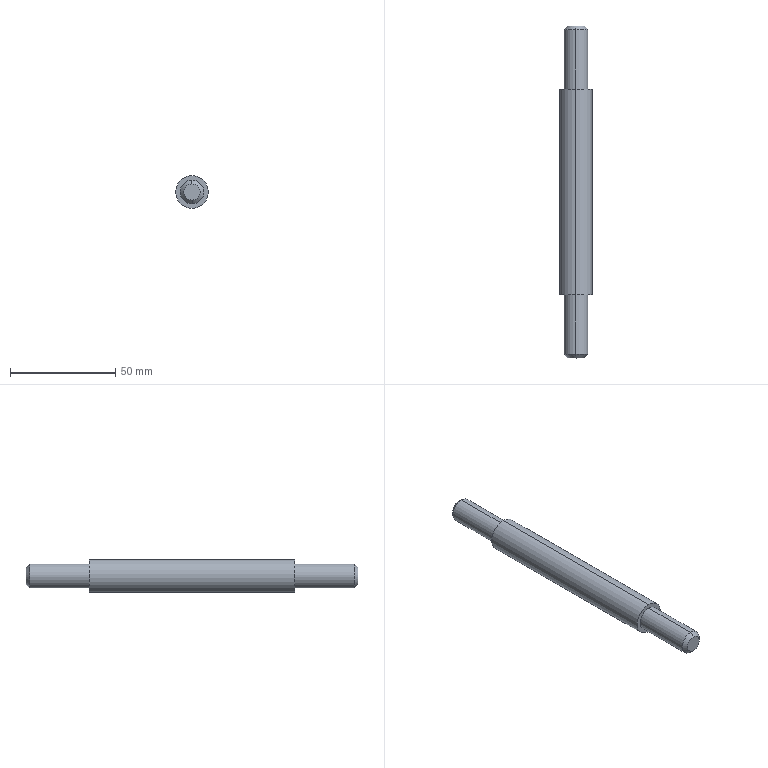Part | STEP file | Scale factor 1[3] | 1 solid | 14 faces | box 15.6 x 157.8 x 15.6 mm | volume 24713 mm3 | cylinder 6 | cone 4 | plane 4 | commonest cylinder face diameters 11.4 x4 15.6 x2
STEP:
#1=CARTESIAN_POINT('',(-699.838,-243.473,3234.6));
#2=VERTEX_POINT('',#1);
#3=CARTESIAN_POINT('',(-699.838,-243.473,3242.4));
#4=VERTEX_POINT('',#3);
#5=CARTESIAN_POINT('',(-699.838,-243.473,3238.5));
#6=DIRECTION('',(0.,1.,0.));
#7=DIRECTION('',(0.000000001,0.,-1.));
#8=AXIS2_PLACEMENT_3D('',#5,#6,#7);
#9=CIRCLE('',#8,3.9);
#10=EDGE_CURVE('',#2,#4,#9,.T.);
#11=ORIENTED_EDGE('',*,*,#10,.F.);
#12=CARTESIAN_POINT('',(-699.838,-245.273,3232.8));
#13=VERTEX_POINT('',#12);
#14=CARTESIAN_POINT('',(-699.838,-243.473,3234.6));
#15=DIRECTION('',(-0.000000001,0.7071,0.7071));
#16=VECTOR('',#15,1000.);
#17=LINE('',#14,#16);
#18=EDGE_CURVE('',#13,#2,#17,.T.);
#19=ORIENTED_EDGE('',*,*,#18,.F.);
#20=CARTESIAN_POINT('',(-699.838,-245.273,3244.2));
#21=VERTEX_POINT('',#20);
#22=CARTESIAN_POINT('',(-699.838,-245.273,3238.5));
#23=DIRECTION('',(0.,-1.,0.));
#24=DIRECTION('',(0.000000001,0.,-1.));
#25=AXIS2_PLACEMENT_3D('',#22,#23,#24);
#26=CIRCLE('',#25,5.7);
#27=EDGE_CURVE('',#21,#13,#26,.T.);
#28=ORIENTED_EDGE('',*,*,#27,.F.);
#29=CARTESIAN_POINT('',(-699.838,-243.473,3242.4));
#30=DIRECTION('',(0.000000001,0.7071,-0.7071));
#31=VECTOR('',#30,1000.);
#32=LINE('',#29,#31);
#33=EDGE_CURVE('',#21,#4,#32,.T.);
#34=ORIENTED_EDGE('',*,*,#33,.T.);
#35=EDGE_LOOP('',(#11,#19,#28,#34));
#36=FACE_OUTER_BOUND('',#35,.T.);
#37=CARTESIAN_POINT('',(-699.838,-243.473,3238.5));
#38=DIRECTION('',(0.,-1.,0.));
#39=DIRECTION('',(0.000000001,0.,-1.));
#40=AXIS2_PLACEMENT_3D('',#37,#38,#39);
#41=CONICAL_SURFACE('',#40,3.9,0.7854);
#42=ADVANCED_FACE('',(#36),#41,.T.);
#43=CARTESIAN_POINT('',(-699.838,-401.273,3242.4));
#44=VERTEX_POINT('',#43);
#45=CARTESIAN_POINT('',(-699.838,-401.273,3234.6));
#46=VERTEX_POINT('',#45);
#47=CARTESIAN_POINT('',(-699.838,-401.273,3238.5));
#48=DIRECTION('',(0.,-1.,0.));
#49=DIRECTION('',(-0.000000001,0.,1.));
#50=AXIS2_PLACEMENT_3D('',#47,#48,#49);
#51=CIRCLE('',#50,3.9);
#52=EDGE_CURVE('',#44,#46,#51,.T.);
#53=ORIENTED_EDGE('',*,*,#52,.F.);
#54=CARTESIAN_POINT('',(-699.838,-399.473,3244.2));
#55=VERTEX_POINT('',#54);
#56=CARTESIAN_POINT('',(-699.838,-401.273,3242.4));
#57=DIRECTION('',(-0.000000001,0.7071,0.7071));
#58=VECTOR('',#57,1000.);
#59=LINE('',#56,#58);
#60=EDGE_CURVE('',#44,#55,#59,.T.);
#61=ORIENTED_EDGE('',*,*,#60,.T.);
#62=CARTESIAN_POINT('',(-699.838,-399.473,3232.8));
#63=VERTEX_POINT('',#62);
#64=CARTESIAN_POINT('',(-699.838,-399.473,3238.5));
#65=DIRECTION('',(0.,1.,0.));
#66=DIRECTION('',(-0.000000001,0.,1.));
#67=AXIS2_PLACEMENT_3D('',#64,#65,#66);
#68=CIRCLE('',#67,5.7);
#69=EDGE_CURVE('',#63,#55,#68,.T.);
#70=ORIENTED_EDGE('',*,*,#69,.F.);
#71=CARTESIAN_POINT('',(-699.838,-401.273,3234.6));
#72=DIRECTION('',(0.000000001,0.7071,-0.7071));
#73=VECTOR('',#72,1000.);
#74=LINE('',#71,#73);
#75=EDGE_CURVE('',#46,#63,#74,.T.);
#76=ORIENTED_EDGE('',*,*,#75,.F.);
#77=EDGE_LOOP('',(#53,#61,#70,#76));
#78=FACE_OUTER_BOUND('',#77,.T.);
#79=CARTESIAN_POINT('',(-699.838,-401.273,3238.5));
#80=DIRECTION('',(0.,1.,0.));
#81=DIRECTION('',(-0.000000001,0.,1.));
#82=AXIS2_PLACEMENT_3D('',#79,#80,#81);
#83=CONICAL_SURFACE('',#82,3.9,0.7854);
#84=ADVANCED_FACE('',(#78),#83,.T.);
#85=ORIENTED_EDGE('',*,*,#69,.T.);
#86=CARTESIAN_POINT('',(-699.838,-371.273,3244.2));
#87=VERTEX_POINT('',#86);
#88=CARTESIAN_POINT('',(-699.838,-401.273,3244.2));
#89=DIRECTION('',(0.,1.,0.));
#90=VECTOR('',#89,1000.);
#91=LINE('',#88,#90);
#92=EDGE_CURVE('',#55,#87,#91,.T.);
#93=ORIENTED_EDGE('',*,*,#92,.T.);
#94=CARTESIAN_POINT('',(-699.838,-371.273,3232.8));
#95=VERTEX_POINT('',#94);
#96=CARTESIAN_POINT('',(-699.838,-371.273,3238.5));
#97=DIRECTION('',(0.,-1.,0.));
#98=DIRECTION('',(0.000000001,0.,-1.));
#99=AXIS2_PLACEMENT_3D('',#96,#97,#98);
#100=CIRCLE('',#99,5.7);
#101=EDGE_CURVE('',#87,#95,#100,.T.);
#102=ORIENTED_EDGE('',*,*,#101,.T.);
#103=CARTESIAN_POINT('',(-699.838,-401.273,3232.8));
#104=DIRECTION('',(0.,1.,0.));
#105=VECTOR('',#104,1000.);
#106=LINE('',#103,#105);
#107=EDGE_CURVE('',#63,#95,#106,.T.);
#108=ORIENTED_EDGE('',*,*,#107,.F.);
#109=EDGE_LOOP('',(#85,#93,#102,#108));
#110=FACE_OUTER_BOUND('',#109,.T.);
#111=CARTESIAN_POINT('',(-699.838,-401.273,3238.5));
#112=DIRECTION('',(0.,1.,0.));
#113=DIRECTION('',(-0.000000001,0.,1.));
#114=AXIS2_PLACEMENT_3D('',#111,#112,#113);
#115=CYLINDRICAL_SURFACE('',#114,5.7);
#116=ADVANCED_FACE('',(#110),#115,.T.);
#117=ORIENTED_EDGE('',*,*,#27,.T.);
#118=CARTESIAN_POINT('',(-699.838,-273.473,3232.8));
#119=VERTEX_POINT('',#118);
#120=CARTESIAN_POINT('',(-699.838,-243.473,3232.8));
#121=DIRECTION('',(0.,1.,0.));
#122=VECTOR('',#121,1000.);
#123=LINE('',#120,#122);
#124=EDGE_CURVE('',#119,#13,#123,.T.);
#125=ORIENTED_EDGE('',*,*,#124,.F.);
#126=CARTESIAN_POINT('',(-699.838,-273.473,3244.2));
#127=VERTEX_POINT('',#126);
#128=CARTESIAN_POINT('',(-699.838,-273.473,3238.5));
#129=DIRECTION('',(0.,1.,0.));
#130=DIRECTION('',(0.000000001,0.,-1.));
#131=AXIS2_PLACEMENT_3D('',#128,#129,#130);
#132=CIRCLE('',#131,5.7);
#133=EDGE_CURVE('',#119,#127,#132,.T.);
#134=ORIENTED_EDGE('',*,*,#133,.T.);
#135=CARTESIAN_POINT('',(-699.838,-243.473,3244.2));
#136=DIRECTION('',(0.,1.,0.));
#137=VECTOR('',#136,1000.);
#138=LINE('',#135,#137);
#139=EDGE_CURVE('',#127,#21,#138,.T.);
#140=ORIENTED_EDGE('',*,*,#139,.T.);
#141=EDGE_LOOP('',(#117,#125,#134,#140));
#142=FACE_OUTER_BOUND('',#141,.T.);
#143=CARTESIAN_POINT('',(-699.838,-243.473,3238.5));
#144=DIRECTION('',(0.,-1.,0.));
#145=DIRECTION('',(0.000000001,0.,-1.));
#146=AXIS2_PLACEMENT_3D('',#143,#144,#145);
#147=CYLINDRICAL_SURFACE('',#146,5.7);
#148=ADVANCED_FACE('',(#142),#147,.T.);
#149=CARTESIAN_POINT('',(-699.838,-273.473,3230.7));
#150=VERTEX_POINT('',#149);
#151=CARTESIAN_POINT('',(-699.838,-273.473,3246.3));
#152=VERTEX_POINT('',#151);
#153=CARTESIAN_POINT('',(-699.838,-273.473,3238.5));
#154=DIRECTION('',(0.,1.,0.));
#155=DIRECTION('',(0.000000001,0.,-1.));
#156=AXIS2_PLACEMENT_3D('',#153,#154,#155);
#157=CIRCLE('',#156,7.8);
#158=EDGE_CURVE('',#150,#152,#157,.T.);
#159=ORIENTED_EDGE('',*,*,#158,.F.);
#160=CARTESIAN_POINT('',(-699.838,-371.273,3230.7));
#161=VERTEX_POINT('',#160);
#162=CARTESIAN_POINT('',(-699.838,-273.473,3230.7));
#163=DIRECTION('',(0.,1.,0.));
#164=VECTOR('',#163,1000.);
#165=LINE('',#162,#164);
#166=EDGE_CURVE('',#161,#150,#165,.T.);
#167=ORIENTED_EDGE('',*,*,#166,.F.);
#168=CARTESIAN_POINT('',(-699.838,-371.273,3246.3));
#169=VERTEX_POINT('',#168);
#170=CARTESIAN_POINT('',(-699.838,-371.273,3238.5));
#171=DIRECTION('',(0.,1.,0.));
#172=DIRECTION('',(0.000000001,0.,-1.));
#173=AXIS2_PLACEMENT_3D('',#170,#171,#172);
#174=CIRCLE('',#173,7.8);
#175=EDGE_CURVE('',#161,#169,#174,.T.);
#176=ORIENTED_EDGE('',*,*,#175,.T.);
#177=CARTESIAN_POINT('',(-699.838,-273.473,3246.3));
#178=DIRECTION('',(0.,1.,0.));
#179=VECTOR('',#178,1000.);
#180=LINE('',#177,#179);
#181=EDGE_CURVE('',#169,#152,#180,.T.);
#182=ORIENTED_EDGE('',*,*,#181,.T.);
#183=EDGE_LOOP('',(#159,#167,#176,#182));
#184=FACE_OUTER_BOUND('',#183,.T.);
#185=CARTESIAN_POINT('',(-699.838,-273.473,3238.5));
#186=DIRECTION('',(0.,-1.,0.));
#187=DIRECTION('',(0.000000001,0.,-1.));
#188=AXIS2_PLACEMENT_3D('',#185,#186,#187);
#189=CYLINDRICAL_SURFACE('',#188,7.8);
#190=ADVANCED_FACE('',(#184),#189,.T.);
#191=ORIENTED_EDGE('',*,*,#166,.T.);
#192=CARTESIAN_POINT('',(-699.838,-273.473,3238.5));
#193=DIRECTION('',(0.,1.,0.));
#194=DIRECTION('',(0.000000001,0.,-1.));
#195=AXIS2_PLACEMENT_3D('',#192,#193,#194);
#196=CIRCLE('',#195,7.8);
#197=EDGE_CURVE('',#152,#150,#196,.T.);
#198=ORIENTED_EDGE('',*,*,#197,.F.);
#199=ORIENTED_EDGE('',*,*,#181,.F.);
#200=CARTESIAN_POINT('',(-699.838,-371.273,3238.5));
#201=DIRECTION('',(0.,1.,0.));
#202=DIRECTION('',(0.000000001,0.,-1.));
#203=AXIS2_PLACEMENT_3D('',#200,#201,#202);
#204=CIRCLE('',#203,7.8);
#205=EDGE_CURVE('',#169,#161,#204,.T.);
#206=ORIENTED_EDGE('',*,*,#205,.T.);
#207=EDGE_LOOP('',(#191,#198,#199,#206));
#208=FACE_OUTER_BOUND('',#207,.T.);
#209=CARTESIAN_POINT('',(-699.838,-273.473,3238.5));
#210=DIRECTION('',(0.,-1.,0.));
#211=DIRECTION('',(0.000000001,0.,-1.));
#212=AXIS2_PLACEMENT_3D('',#209,#210,#211);
#213=CYLINDRICAL_SURFACE('',#212,7.8);
#214=ADVANCED_FACE('',(#208),#213,.T.);
#215=CARTESIAN_POINT('',(-699.838,-273.473,3238.5));
#216=DIRECTION('',(0.,1.,0.));
#217=DIRECTION('',(0.000000001,0.,-1.));
#218=AXIS2_PLACEMENT_3D('',#215,#216,#217);
#219=CIRCLE('',#218,5.7);
#220=EDGE_CURVE('',#127,#119,#219,.T.);
#221=ORIENTED_EDGE('',*,*,#220,.F.);
#222=ORIENTED_EDGE('',*,*,#133,.F.);
#223=EDGE_LOOP('',(#221,#222));
#224=FACE_BOUND('',#223,.T.);
#225=ORIENTED_EDGE('',*,*,#197,.T.);
#226=ORIENTED_EDGE('',*,*,#158,.T.);
#227=EDGE_LOOP('',(#225,#226));
#228=FACE_OUTER_BOUND('',#227,.T.);
#229=CARTESIAN_POINT('',(-699.838,-273.473,3238.5));
#230=DIRECTION('',(0.,1.,0.));
#231=DIRECTION('',(-0.000000001,0.,1.));
#232=AXIS2_PLACEMENT_3D('',#229,#230,#231);
#233=PLANE('',#232);
#234=ADVANCED_FACE('',(#224,#228),#233,.T.);
#235=CARTESIAN_POINT('',(-699.838,-371.273,3238.5));
#236=DIRECTION('',(0.,-1.,0.));
#237=DIRECTION('',(0.000000001,0.,-1.));
#238=AXIS2_PLACEMENT_3D('',#235,#236,#237);
#239=CIRCLE('',#238,5.7);
#240=EDGE_CURVE('',#95,#87,#239,.T.);
#241=ORIENTED_EDGE('',*,*,#240,.F.);
#242=ORIENTED_EDGE('',*,*,#101,.F.);
#243=EDGE_LOOP('',(#241,#242));
#244=FACE_BOUND('',#243,.T.);
#245=ORIENTED_EDGE('',*,*,#205,.F.);
#246=ORIENTED_EDGE('',*,*,#175,.F.);
#247=EDGE_LOOP('',(#245,#246));
#248=FACE_OUTER_BOUND('',#247,.T.);
#249=CARTESIAN_POINT('',(-699.838,-371.273,3238.5));
#250=DIRECTION('',(0.,1.,0.));
#251=DIRECTION('',(-0.000000001,0.,1.));
#252=AXIS2_PLACEMENT_3D('',#249,#250,#251);
#253=PLANE('',#252);
#254=ADVANCED_FACE('',(#244,#248),#253,.F.);
#255=ORIENTED_EDGE('',*,*,#124,.T.);
#256=CARTESIAN_POINT('',(-699.838,-245.273,3238.5));
#257=DIRECTION('',(0.,-1.,0.));
#258=DIRECTION('',(0.000000001,0.,-1.));
#259=AXIS2_PLACEMENT_3D('',#256,#257,#258);
#260=CIRCLE('',#259,5.7);
#261=EDGE_CURVE('',#13,#21,#260,.T.);
#262=ORIENTED_EDGE('',*,*,#261,.T.);
#263=ORIENTED_EDGE('',*,*,#139,.F.);
#264=ORIENTED_EDGE('',*,*,#220,.T.);
#265=EDGE_LOOP('',(#255,#262,#263,#264));
#266=FACE_OUTER_BOUND('',#265,.T.);
#267=CARTESIAN_POINT('',(-699.838,-243.473,3238.5));
#268=DIRECTION('',(0.,-1.,0.));
#269=DIRECTION('',(0.000000001,0.,-1.));
#270=AXIS2_PLACEMENT_3D('',#267,#268,#269);
#271=CYLINDRICAL_SURFACE('',#270,5.7);
#272=ADVANCED_FACE('',(#266),#271,.T.);
#273=CARTESIAN_POINT('',(-699.838,-243.473,3238.5));
#274=DIRECTION('',(0.,1.,0.));
#275=DIRECTION('',(0.000000001,0.,-1.));
#276=AXIS2_PLACEMENT_3D('',#273,#274,#275);
#277=CIRCLE('',#276,3.9);
#278=EDGE_CURVE('',#4,#2,#277,.T.);
#279=ORIENTED_EDGE('',*,*,#278,.T.);
#280=ORIENTED_EDGE('',*,*,#10,.T.);
#281=EDGE_LOOP('',(#279,#280));
#282=FACE_OUTER_BOUND('',#281,.T.);
#283=CARTESIAN_POINT('',(-699.838,-243.473,3238.5));
#284=DIRECTION('',(0.,1.,0.));
#285=DIRECTION('',(-0.000000001,0.,1.));
#286=AXIS2_PLACEMENT_3D('',#283,#284,#285);
#287=PLANE('',#286);
#288=ADVANCED_FACE('',(#282),#287,.T.);
#289=ORIENTED_EDGE('',*,*,#92,.F.);
#290=CARTESIAN_POINT('',(-699.838,-399.473,3238.5));
#291=DIRECTION('',(0.,1.,0.));
#292=DIRECTION('',(-0.000000001,0.,1.));
#293=AXIS2_PLACEMENT_3D('',#290,#291,#292);
#294=CIRCLE('',#293,5.7);
#295=EDGE_CURVE('',#55,#63,#294,.T.);
#296=ORIENTED_EDGE('',*,*,#295,.T.);
#297=ORIENTED_EDGE('',*,*,#107,.T.);
#298=ORIENTED_EDGE('',*,*,#240,.T.);
#299=EDGE_LOOP('',(#289,#296,#297,#298));
#300=FACE_OUTER_BOUND('',#299,.T.);
#301=CARTESIAN_POINT('',(-699.838,-401.273,3238.5));
#302=DIRECTION('',(0.,1.,0.));
#303=DIRECTION('',(-0.000000001,0.,1.));
#304=AXIS2_PLACEMENT_3D('',#301,#302,#303);
#305=CYLINDRICAL_SURFACE('',#304,5.7);
#306=ADVANCED_FACE('',(#300),#305,.T.);
#307=CARTESIAN_POINT('',(-699.838,-401.273,3238.5));
#308=DIRECTION('',(0.,-1.,0.));
#309=DIRECTION('',(-0.000000001,0.,1.));
#310=AXIS2_PLACEMENT_3D('',#307,#308,#309);
#311=CIRCLE('',#310,3.9);
#312=EDGE_CURVE('',#46,#44,#311,.T.);
#313=ORIENTED_EDGE('',*,*,#312,.T.);
#314=ORIENTED_EDGE('',*,*,#52,.T.);
#315=EDGE_LOOP('',(#313,#314));
#316=FACE_OUTER_BOUND('',#315,.T.);
#317=CARTESIAN_POINT('',(-699.838,-401.273,3238.5));
#318=DIRECTION('',(0.,-1.,0.));
#319=DIRECTION('',(0.000000001,0.,-1.));
#320=AXIS2_PLACEMENT_3D('',#317,#318,#319);
#321=PLANE('',#320);
#322=ADVANCED_FACE('',(#316),#321,.T.);
#323=ORIENTED_EDGE('',*,*,#60,.F.);
#324=ORIENTED_EDGE('',*,*,#312,.F.);
#325=ORIENTED_EDGE('',*,*,#75,.T.);
#326=ORIENTED_EDGE('',*,*,#295,.F.);
#327=EDGE_LOOP('',(#323,#324,#325,#326));
#328=FACE_OUTER_BOUND('',#327,.T.);
#329=CARTESIAN_POINT('',(-699.838,-401.273,3238.5));
#330=DIRECTION('',(0.,1.,0.));
#331=DIRECTION('',(-0.000000001,0.,1.));
#332=AXIS2_PLACEMENT_3D('',#329,#330,#331);
#333=CONICAL_SURFACE('',#332,3.9,0.7854);
#334=ADVANCED_FACE('',(#328),#333,.T.);
#335=ORIENTED_EDGE('',*,*,#18,.T.);
#336=ORIENTED_EDGE('',*,*,#278,.F.);
#337=ORIENTED_EDGE('',*,*,#33,.F.);
#338=ORIENTED_EDGE('',*,*,#261,.F.);
#339=EDGE_LOOP('',(#335,#336,#337,#338));
#340=FACE_OUTER_BOUND('',#339,.T.);
#341=CARTESIAN_POINT('',(-699.838,-243.473,3238.5));
#342=DIRECTION('',(0.,-1.,0.));
#343=DIRECTION('',(0.000000001,0.,-1.));
#344=AXIS2_PLACEMENT_3D('',#341,#342,#343);
#345=CONICAL_SURFACE('',#344,3.9,0.7854);
#346=ADVANCED_FACE('',(#340),#345,.T.);
#347=CLOSED_SHELL('',(#42,#84,#116,#148,#190,#214,#234,#254,#272,#288,#306,#322,#334,#346));
#348=MANIFOLD_SOLID_BREP('',#347);
#349=CARTESIAN_POINT('',(0.,0.,0.));
#350=DIRECTION('',(0.,0.,1.));
#351=DIRECTION('',(1.,0.,0.));
#352=AXIS2_PLACEMENT_3D('',#349,#350,#351);
#353=(LENGTH_UNIT()NAMED_UNIT(*)SI_UNIT(.MILLI.,.METRE.));
#354=UNCERTAINTY_MEASURE_WITH_UNIT(LENGTH_MEASURE(0.00001),#353,'','');
#355=(NAMED_UNIT(*)PLANE_ANGLE_UNIT()SI_UNIT($,.RADIAN.));
#356=(NAMED_UNIT(*)SI_UNIT($,.STERADIAN.)SOLID_ANGLE_UNIT());
#357=(GEOMETRIC_REPRESENTATION_CONTEXT(3)GLOBAL_UNCERTAINTY_ASSIGNED_CONTEXT((#354))GLOBAL_UNIT_ASSIGNED_CONTEXT((#353,#355,#356))REPRESENTATION_CONTEXT('',''));
#358=ADVANCED_BREP_SHAPE_REPRESENTATION('',(#348,#352),#357);